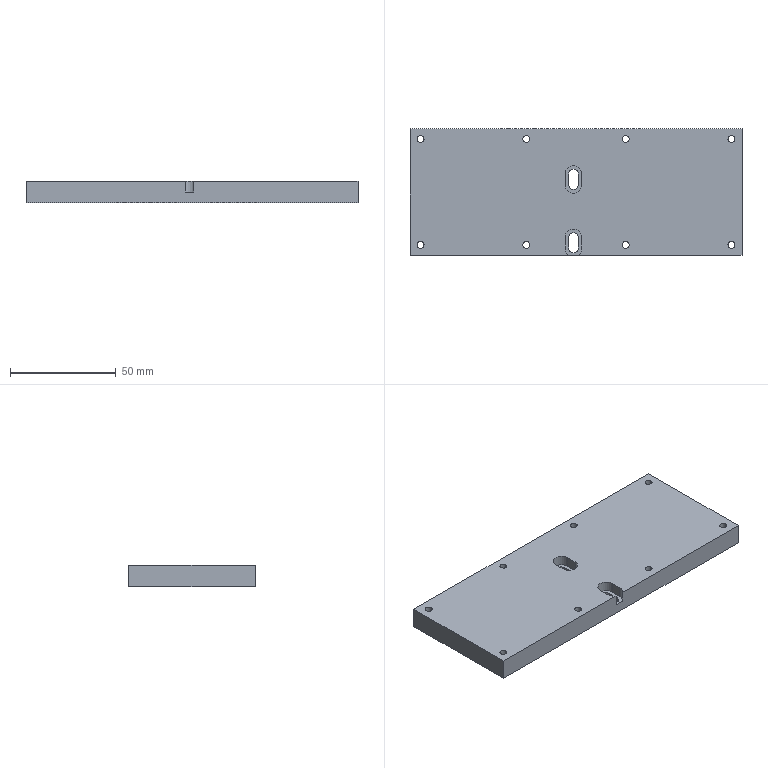Part | STEP file | 04-02-05 adjustment platform base plate | 1 solid | 41 faces | box 157 x 60 x 10 mm | volume 92232 mm3 | cylinder 25 | plane 16 | commonest cylinder face diameters 3.3 x16 8 x5 4.5 x4
STEP:
#1=CARTESIAN_POINT('',(71.85,25.,0.));
#2=VERTEX_POINT('',#1);
#3=CARTESIAN_POINT('',(75.15,25.,0.));
#4=VERTEX_POINT('',#3);
#5=CARTESIAN_POINT('',(73.5,25.,0.));
#6=DIRECTION('',(0.,0.,1.));
#7=DIRECTION('',(1.,0.,0.));
#8=AXIS2_PLACEMENT_3D('',#5,#6,#7);
#9=CIRCLE('',#8,1.65);
#10=EDGE_CURVE('',#2,#4,#9,.T.);
#11=ORIENTED_EDGE('',*,*,#10,.F.);
#12=CARTESIAN_POINT('',(71.85,25.,10.));
#13=VERTEX_POINT('',#12);
#14=CARTESIAN_POINT('',(71.85,25.,10.));
#15=DIRECTION('',(0.,0.,1.));
#16=VECTOR('',#15,1000.);
#17=LINE('',#14,#16);
#18=EDGE_CURVE('',#2,#13,#17,.T.);
#19=ORIENTED_EDGE('',*,*,#18,.T.);
#20=CARTESIAN_POINT('',(75.15,25.,10.));
#21=VERTEX_POINT('',#20);
#22=CARTESIAN_POINT('',(73.5,25.,10.));
#23=DIRECTION('',(0.,0.,1.));
#24=DIRECTION('',(1.,0.,0.));
#25=AXIS2_PLACEMENT_3D('',#22,#23,#24);
#26=CIRCLE('',#25,1.65);
#27=EDGE_CURVE('',#13,#21,#26,.T.);
#28=ORIENTED_EDGE('',*,*,#27,.T.);
#29=CARTESIAN_POINT('',(75.15,25.,10.));
#30=DIRECTION('',(0.,0.,1.));
#31=VECTOR('',#30,1000.);
#32=LINE('',#29,#31);
#33=EDGE_CURVE('',#4,#21,#32,.T.);
#34=ORIENTED_EDGE('',*,*,#33,.F.);
#35=EDGE_LOOP('',(#11,#19,#28,#34));
#36=FACE_OUTER_BOUND('',#35,.T.);
#37=CARTESIAN_POINT('',(73.5,25.,10.));
#38=DIRECTION('',(0.,0.,1.));
#39=DIRECTION('',(1.,0.,0.));
#40=AXIS2_PLACEMENT_3D('',#37,#38,#39);
#41=CYLINDRICAL_SURFACE('',#40,1.65);
#42=ADVANCED_FACE('',(#36),#41,.F.);
#43=CARTESIAN_POINT('',(21.85,-25.,0.));
#44=VERTEX_POINT('',#43);
#45=CARTESIAN_POINT('',(25.15,-25.,0.));
#46=VERTEX_POINT('',#45);
#47=CARTESIAN_POINT('',(23.5,-25.,0.));
#48=DIRECTION('',(0.,0.,1.));
#49=DIRECTION('',(1.,0.,0.));
#50=AXIS2_PLACEMENT_3D('',#47,#48,#49);
#51=CIRCLE('',#50,1.65);
#52=EDGE_CURVE('',#44,#46,#51,.T.);
#53=ORIENTED_EDGE('',*,*,#52,.F.);
#54=CARTESIAN_POINT('',(21.85,-25.,10.));
#55=VERTEX_POINT('',#54);
#56=CARTESIAN_POINT('',(21.85,-25.,10.));
#57=DIRECTION('',(0.,0.,1.));
#58=VECTOR('',#57,1000.);
#59=LINE('',#56,#58);
#60=EDGE_CURVE('',#44,#55,#59,.T.);
#61=ORIENTED_EDGE('',*,*,#60,.T.);
#62=CARTESIAN_POINT('',(25.15,-25.,10.));
#63=VERTEX_POINT('',#62);
#64=CARTESIAN_POINT('',(23.5,-25.,10.));
#65=DIRECTION('',(0.,0.,1.));
#66=DIRECTION('',(1.,0.,0.));
#67=AXIS2_PLACEMENT_3D('',#64,#65,#66);
#68=CIRCLE('',#67,1.65);
#69=EDGE_CURVE('',#55,#63,#68,.T.);
#70=ORIENTED_EDGE('',*,*,#69,.T.);
#71=CARTESIAN_POINT('',(25.15,-25.,10.));
#72=DIRECTION('',(0.,0.,1.));
#73=VECTOR('',#72,1000.);
#74=LINE('',#71,#73);
#75=EDGE_CURVE('',#46,#63,#74,.T.);
#76=ORIENTED_EDGE('',*,*,#75,.F.);
#77=EDGE_LOOP('',(#53,#61,#70,#76));
#78=FACE_OUTER_BOUND('',#77,.T.);
#79=CARTESIAN_POINT('',(23.5,-25.,10.));
#80=DIRECTION('',(0.,0.,1.));
#81=DIRECTION('',(1.,0.,0.));
#82=AXIS2_PLACEMENT_3D('',#79,#80,#81);
#83=CYLINDRICAL_SURFACE('',#82,1.65);
#84=ADVANCED_FACE('',(#78),#83,.F.);
#85=CARTESIAN_POINT('',(71.85,-25.,0.));
#86=VERTEX_POINT('',#85);
#87=CARTESIAN_POINT('',(75.15,-25.,0.));
#88=VERTEX_POINT('',#87);
#89=CARTESIAN_POINT('',(73.5,-25.,0.));
#90=DIRECTION('',(0.,0.,1.));
#91=DIRECTION('',(1.,0.,0.));
#92=AXIS2_PLACEMENT_3D('',#89,#90,#91);
#93=CIRCLE('',#92,1.65);
#94=EDGE_CURVE('',#86,#88,#93,.T.);
#95=ORIENTED_EDGE('',*,*,#94,.F.);
#96=CARTESIAN_POINT('',(71.85,-25.,10.));
#97=VERTEX_POINT('',#96);
#98=CARTESIAN_POINT('',(71.85,-25.,10.));
#99=DIRECTION('',(0.,0.,1.));
#100=VECTOR('',#99,1000.);
#101=LINE('',#98,#100);
#102=EDGE_CURVE('',#86,#97,#101,.T.);
#103=ORIENTED_EDGE('',*,*,#102,.T.);
#104=CARTESIAN_POINT('',(75.15,-25.,10.));
#105=VERTEX_POINT('',#104);
#106=CARTESIAN_POINT('',(73.5,-25.,10.));
#107=DIRECTION('',(0.,0.,1.));
#108=DIRECTION('',(1.,0.,0.));
#109=AXIS2_PLACEMENT_3D('',#106,#107,#108);
#110=CIRCLE('',#109,1.65);
#111=EDGE_CURVE('',#97,#105,#110,.T.);
#112=ORIENTED_EDGE('',*,*,#111,.T.);
#113=CARTESIAN_POINT('',(75.15,-25.,10.));
#114=DIRECTION('',(0.,0.,1.));
#115=VECTOR('',#114,1000.);
#116=LINE('',#113,#115);
#117=EDGE_CURVE('',#88,#105,#116,.T.);
#118=ORIENTED_EDGE('',*,*,#117,.F.);
#119=EDGE_LOOP('',(#95,#103,#112,#118));
#120=FACE_OUTER_BOUND('',#119,.T.);
#121=CARTESIAN_POINT('',(73.5,-25.,10.));
#122=DIRECTION('',(0.,0.,1.));
#123=DIRECTION('',(1.,0.,0.));
#124=AXIS2_PLACEMENT_3D('',#121,#122,#123);
#125=CYLINDRICAL_SURFACE('',#124,1.65);
#126=ADVANCED_FACE('',(#120),#125,.F.);
#127=CARTESIAN_POINT('',(21.85,25.,0.));
#128=VERTEX_POINT('',#127);
#129=CARTESIAN_POINT('',(25.15,25.,0.));
#130=VERTEX_POINT('',#129);
#131=CARTESIAN_POINT('',(23.5,25.,0.));
#132=DIRECTION('',(0.,0.,1.));
#133=DIRECTION('',(1.,0.,0.));
#134=AXIS2_PLACEMENT_3D('',#131,#132,#133);
#135=CIRCLE('',#134,1.65);
#136=EDGE_CURVE('',#128,#130,#135,.T.);
#137=ORIENTED_EDGE('',*,*,#136,.F.);
#138=CARTESIAN_POINT('',(21.85,25.,10.));
#139=VERTEX_POINT('',#138);
#140=CARTESIAN_POINT('',(21.85,25.,10.));
#141=DIRECTION('',(0.,0.,1.));
#142=VECTOR('',#141,1000.);
#143=LINE('',#140,#142);
#144=EDGE_CURVE('',#128,#139,#143,.T.);
#145=ORIENTED_EDGE('',*,*,#144,.T.);
#146=CARTESIAN_POINT('',(25.15,25.,10.));
#147=VERTEX_POINT('',#146);
#148=CARTESIAN_POINT('',(23.5,25.,10.));
#149=DIRECTION('',(0.,0.,1.));
#150=DIRECTION('',(1.,0.,0.));
#151=AXIS2_PLACEMENT_3D('',#148,#149,#150);
#152=CIRCLE('',#151,1.65);
#153=EDGE_CURVE('',#139,#147,#152,.T.);
#154=ORIENTED_EDGE('',*,*,#153,.T.);
#155=CARTESIAN_POINT('',(25.15,25.,10.));
#156=DIRECTION('',(0.,0.,1.));
#157=VECTOR('',#156,1000.);
#158=LINE('',#155,#157);
#159=EDGE_CURVE('',#130,#147,#158,.T.);
#160=ORIENTED_EDGE('',*,*,#159,.F.);
#161=EDGE_LOOP('',(#137,#145,#154,#160));
#162=FACE_OUTER_BOUND('',#161,.T.);
#163=CARTESIAN_POINT('',(23.5,25.,10.));
#164=DIRECTION('',(0.,0.,1.));
#165=DIRECTION('',(1.,0.,0.));
#166=AXIS2_PLACEMENT_3D('',#163,#164,#165);
#167=CYLINDRICAL_SURFACE('',#166,1.65);
#168=ADVANCED_FACE('',(#162),#167,.F.);
#169=CARTESIAN_POINT('',(-75.15,25.,0.));
#170=VERTEX_POINT('',#169);
#171=CARTESIAN_POINT('',(-71.85,25.,0.));
#172=VERTEX_POINT('',#171);
#173=CARTESIAN_POINT('',(-73.5,25.,0.));
#174=DIRECTION('',(0.,0.,1.));
#175=DIRECTION('',(1.,0.,0.));
#176=AXIS2_PLACEMENT_3D('',#173,#174,#175);
#177=CIRCLE('',#176,1.65);
#178=EDGE_CURVE('',#170,#172,#177,.T.);
#179=ORIENTED_EDGE('',*,*,#178,.F.);
#180=CARTESIAN_POINT('',(-75.15,25.,10.));
#181=VERTEX_POINT('',#180);
#182=CARTESIAN_POINT('',(-75.15,25.,10.));
#183=DIRECTION('',(0.,0.,1.));
#184=VECTOR('',#183,1000.);
#185=LINE('',#182,#184);
#186=EDGE_CURVE('',#170,#181,#185,.T.);
#187=ORIENTED_EDGE('',*,*,#186,.T.);
#188=CARTESIAN_POINT('',(-71.85,25.,10.));
#189=VERTEX_POINT('',#188);
#190=CARTESIAN_POINT('',(-73.5,25.,10.));
#191=DIRECTION('',(0.,0.,1.));
#192=DIRECTION('',(1.,0.,0.));
#193=AXIS2_PLACEMENT_3D('',#190,#191,#192);
#194=CIRCLE('',#193,1.65);
#195=EDGE_CURVE('',#181,#189,#194,.T.);
#196=ORIENTED_EDGE('',*,*,#195,.T.);
#197=CARTESIAN_POINT('',(-71.85,25.,10.));
#198=DIRECTION('',(0.,0.,1.));
#199=VECTOR('',#198,1000.);
#200=LINE('',#197,#199);
#201=EDGE_CURVE('',#172,#189,#200,.T.);
#202=ORIENTED_EDGE('',*,*,#201,.F.);
#203=EDGE_LOOP('',(#179,#187,#196,#202));
#204=FACE_OUTER_BOUND('',#203,.T.);
#205=CARTESIAN_POINT('',(-73.5,25.,10.));
#206=DIRECTION('',(0.,0.,1.));
#207=DIRECTION('',(1.,0.,0.));
#208=AXIS2_PLACEMENT_3D('',#205,#206,#207);
#209=CYLINDRICAL_SURFACE('',#208,1.65);
#210=ADVANCED_FACE('',(#204),#209,.F.);
#211=CARTESIAN_POINT('',(-25.15,25.,0.));
#212=VERTEX_POINT('',#211);
#213=CARTESIAN_POINT('',(-21.85,25.,0.));
#214=VERTEX_POINT('',#213);
#215=CARTESIAN_POINT('',(-23.5,25.,0.));
#216=DIRECTION('',(0.,0.,1.));
#217=DIRECTION('',(1.,0.,0.));
#218=AXIS2_PLACEMENT_3D('',#215,#216,#217);
#219=CIRCLE('',#218,1.65);
#220=EDGE_CURVE('',#212,#214,#219,.T.);
#221=ORIENTED_EDGE('',*,*,#220,.F.);
#222=CARTESIAN_POINT('',(-25.15,25.,10.));
#223=VERTEX_POINT('',#222);
#224=CARTESIAN_POINT('',(-25.15,25.,10.));
#225=DIRECTION('',(0.,0.,1.));
#226=VECTOR('',#225,1000.);
#227=LINE('',#224,#226);
#228=EDGE_CURVE('',#212,#223,#227,.T.);
#229=ORIENTED_EDGE('',*,*,#228,.T.);
#230=CARTESIAN_POINT('',(-21.85,25.,10.));
#231=VERTEX_POINT('',#230);
#232=CARTESIAN_POINT('',(-23.5,25.,10.));
#233=DIRECTION('',(0.,0.,1.));
#234=DIRECTION('',(1.,0.,0.));
#235=AXIS2_PLACEMENT_3D('',#232,#233,#234);
#236=CIRCLE('',#235,1.65);
#237=EDGE_CURVE('',#223,#231,#236,.T.);
#238=ORIENTED_EDGE('',*,*,#237,.T.);
#239=CARTESIAN_POINT('',(-21.85,25.,10.));
#240=DIRECTION('',(0.,0.,1.));
#241=VECTOR('',#240,1000.);
#242=LINE('',#239,#241);
#243=EDGE_CURVE('',#214,#231,#242,.T.);
#244=ORIENTED_EDGE('',*,*,#243,.F.);
#245=EDGE_LOOP('',(#221,#229,#238,#244));
#246=FACE_OUTER_BOUND('',#245,.T.);
#247=CARTESIAN_POINT('',(-23.5,25.,10.));
#248=DIRECTION('',(0.,0.,1.));
#249=DIRECTION('',(1.,0.,0.));
#250=AXIS2_PLACEMENT_3D('',#247,#248,#249);
#251=CYLINDRICAL_SURFACE('',#250,1.65);
#252=ADVANCED_FACE('',(#246),#251,.F.);
#253=CARTESIAN_POINT('',(-75.15,-25.,0.));
#254=VERTEX_POINT('',#253);
#255=CARTESIAN_POINT('',(-71.85,-25.,0.));
#256=VERTEX_POINT('',#255);
#257=CARTESIAN_POINT('',(-73.5,-25.,0.));
#258=DIRECTION('',(0.,0.,1.));
#259=DIRECTION('',(1.,0.,0.));
#260=AXIS2_PLACEMENT_3D('',#257,#258,#259);
#261=CIRCLE('',#260,1.65);
#262=EDGE_CURVE('',#254,#256,#261,.T.);
#263=ORIENTED_EDGE('',*,*,#262,.F.);
#264=CARTESIAN_POINT('',(-75.15,-25.,10.));
#265=VERTEX_POINT('',#264);
#266=CARTESIAN_POINT('',(-75.15,-25.,10.));
#267=DIRECTION('',(0.,0.,1.));
#268=VECTOR('',#267,1000.);
#269=LINE('',#266,#268);
#270=EDGE_CURVE('',#254,#265,#269,.T.);
#271=ORIENTED_EDGE('',*,*,#270,.T.);
#272=CARTESIAN_POINT('',(-71.85,-25.,10.));
#273=VERTEX_POINT('',#272);
#274=CARTESIAN_POINT('',(-73.5,-25.,10.));
#275=DIRECTION('',(0.,0.,1.));
#276=DIRECTION('',(1.,0.,0.));
#277=AXIS2_PLACEMENT_3D('',#274,#275,#276);
#278=CIRCLE('',#277,1.65);
#279=EDGE_CURVE('',#265,#273,#278,.T.);
#280=ORIENTED_EDGE('',*,*,#279,.T.);
#281=CARTESIAN_POINT('',(-71.85,-25.,10.));
#282=DIRECTION('',(0.,0.,1.));
#283=VECTOR('',#282,1000.);
#284=LINE('',#281,#283);
#285=EDGE_CURVE('',#256,#273,#284,.T.);
#286=ORIENTED_EDGE('',*,*,#285,.F.);
#287=EDGE_LOOP('',(#263,#271,#280,#286));
#288=FACE_OUTER_BOUND('',#287,.T.);
#289=CARTESIAN_POINT('',(-73.5,-25.,10.));
#290=DIRECTION('',(0.,0.,1.));
#291=DIRECTION('',(1.,0.,0.));
#292=AXIS2_PLACEMENT_3D('',#289,#290,#291);
#293=CYLINDRICAL_SURFACE('',#292,1.65);
#294=ADVANCED_FACE('',(#288),#293,.F.);
#295=CARTESIAN_POINT('',(-25.15,-25.,0.));
#296=VERTEX_POINT('',#295);
#297=CARTESIAN_POINT('',(-21.85,-25.,0.));
#298=VERTEX_POINT('',#297);
#299=CARTESIAN_POINT('',(-23.5,-25.,0.));
#300=DIRECTION('',(0.,0.,1.));
#301=DIRECTION('',(1.,0.,0.));
#302=AXIS2_PLACEMENT_3D('',#299,#300,#301);
#303=CIRCLE('',#302,1.65);
#304=EDGE_CURVE('',#296,#298,#303,.T.);
#305=ORIENTED_EDGE('',*,*,#304,.F.);
#306=CARTESIAN_POINT('',(-25.15,-25.,10.));
#307=VERTEX_POINT('',#306);
#308=CARTESIAN_POINT('',(-25.15,-25.,10.));
#309=DIRECTION('',(0.,0.,1.));
#310=VECTOR('',#309,1000.);
#311=LINE('',#308,#310);
#312=EDGE_CURVE('',#296,#307,#311,.T.);
#313=ORIENTED_EDGE('',*,*,#312,.T.);
#314=CARTESIAN_POINT('',(-21.85,-25.,10.));
#315=VERTEX_POINT('',#314);
#316=CARTESIAN_POINT('',(-23.5,-25.,10.));
#317=DIRECTION('',(0.,0.,1.));
#318=DIRECTION('',(1.,0.,0.));
#319=AXIS2_PLACEMENT_3D('',#316,#317,#318);
#320=CIRCLE('',#319,1.65);
#321=EDGE_CURVE('',#307,#315,#320,.T.);
#322=ORIENTED_EDGE('',*,*,#321,.T.);
#323=CARTESIAN_POINT('',(-21.85,-25.,10.));
#324=DIRECTION('',(0.,0.,1.));
#325=VECTOR('',#324,1000.);
#326=LINE('',#323,#325);
#327=EDGE_CURVE('',#298,#315,#326,.T.);
#328=ORIENTED_EDGE('',*,*,#327,.F.);
#329=EDGE_LOOP('',(#305,#313,#322,#328));
#330=FACE_OUTER_BOUND('',#329,.T.);
#331=CARTESIAN_POINT('',(-23.5,-25.,10.));
#332=DIRECTION('',(0.,0.,1.));
#333=DIRECTION('',(1.,0.,0.));
#334=AXIS2_PLACEMENT_3D('',#331,#332,#333);
#335=CYLINDRICAL_SURFACE('',#334,1.65);
#336=ADVANCED_FACE('',(#330),#335,.F.);
#337=CARTESIAN_POINT('',(-3.45,-21.5,5.));
#338=VERTEX_POINT('',#337);
#339=CARTESIAN_POINT('',(1.05,-21.5,5.));
#340=VERTEX_POINT('',#339);
#341=CARTESIAN_POINT('',(-1.2,-21.5,5.));
#342=DIRECTION('',(0.,0.,-1.));
#343=DIRECTION('',(1.,0.,0.));
#344=AXIS2_PLACEMENT_3D('',#341,#342,#343);
#345=CIRCLE('',#344,2.25);
#346=EDGE_CURVE('',#338,#340,#345,.T.);
#347=ORIENTED_EDGE('',*,*,#346,.F.);
#348=CARTESIAN_POINT('',(-3.45,-21.5,0.));
#349=VERTEX_POINT('',#348);
#350=CARTESIAN_POINT('',(-3.45,-21.5,0.));
#351=DIRECTION('',(0.,0.,1.));
#352=VECTOR('',#351,1000.);
#353=LINE('',#350,#352);
#354=EDGE_CURVE('',#349,#338,#353,.T.);
#355=ORIENTED_EDGE('',*,*,#354,.F.);
#356=CARTESIAN_POINT('',(1.05,-21.5,0.));
#357=VERTEX_POINT('',#356);
#358=CARTESIAN_POINT('',(-1.2,-21.5,0.));
#359=DIRECTION('',(0.,0.,1.));
#360=DIRECTION('',(1.,0.,0.));
#361=AXIS2_PLACEMENT_3D('',#358,#359,#360);
#362=CIRCLE('',#361,2.25);
#363=EDGE_CURVE('',#357,#349,#362,.T.);
#364=ORIENTED_EDGE('',*,*,#363,.F.);
#365=CARTESIAN_POINT('',(1.05,-21.5,0.));
#366=DIRECTION('',(0.,0.,1.));
#367=VECTOR('',#366,1000.);
#368=LINE('',#365,#367);
#369=EDGE_CURVE('',#357,#340,#368,.T.);
#370=ORIENTED_EDGE('',*,*,#369,.T.);
#371=EDGE_LOOP('',(#347,#355,#364,#370));
#372=FACE_OUTER_BOUND('',#371,.T.);
#373=CARTESIAN_POINT('',(-1.2,-21.5,0.));
#374=DIRECTION('',(0.,0.,1.));
#375=DIRECTION('',(1.,0.,0.));
#376=AXIS2_PLACEMENT_3D('',#373,#374,#375);
#377=CYLINDRICAL_SURFACE('',#376,2.25);
#378=ADVANCED_FACE('',(#372),#377,.F.);
#379=CARTESIAN_POINT('',(1.05,-26.5,5.));
#380=VERTEX_POINT('',#379);
#381=CARTESIAN_POINT('',(1.05,-21.5,5.));
#382=DIRECTION('',(0.,-1.,0.));
#383=VECTOR('',#382,1000.);
#384=LINE('',#381,#383);
#385=EDGE_CURVE('',#340,#380,#384,.T.);
#386=ORIENTED_EDGE('',*,*,#385,.F.);
#387=ORIENTED_EDGE('',*,*,#369,.F.);
#388=CARTESIAN_POINT('',(1.05,-26.5,0.));
#389=VERTEX_POINT('',#388);
#390=CARTESIAN_POINT('',(1.05,-21.5,0.));
#391=DIRECTION('',(0.,1.,0.));
#392=VECTOR('',#391,1000.);
#393=LINE('',#390,#392);
#394=EDGE_CURVE('',#389,#357,#393,.T.);
#395=ORIENTED_EDGE('',*,*,#394,.F.);
#396=CARTESIAN_POINT('',(1.05,-26.5,0.));
#397=DIRECTION('',(0.,0.,1.));
#398=VECTOR('',#397,1000.);
#399=LINE('',#396,#398);
#400=EDGE_CURVE('',#389,#380,#399,.T.);
#401=ORIENTED_EDGE('',*,*,#400,.T.);
#402=EDGE_LOOP('',(#386,#387,#395,#401));
#403=FACE_OUTER_BOUND('',#402,.T.);
#404=CARTESIAN_POINT('',(1.05,-21.5,0.));
#405=DIRECTION('',(1.,0.,0.));
#406=DIRECTION('',(0.,1.,0.));
#407=AXIS2_PLACEMENT_3D('',#404,#405,#406);
#408=PLANE('',#407);
#409=ADVANCED_FACE('',(#403),#408,.F.);
#410=CARTESIAN_POINT('',(-3.45,-26.5,5.));
#411=VERTEX_POINT('',#410);
#412=CARTESIAN_POINT('',(-1.2,-26.5,5.));
#413=DIRECTION('',(0.,0.,-1.));
#414=DIRECTION('',(1.,0.,0.));
#415=AXIS2_PLACEMENT_3D('',#412,#413,#414);
#416=CIRCLE('',#415,2.25);
#417=EDGE_CURVE('',#380,#411,#416,.T.);
#418=ORIENTED_EDGE('',*,*,#417,.F.);
#419=ORIENTED_EDGE('',*,*,#400,.F.);
#420=CARTESIAN_POINT('',(-3.45,-26.5,0.));
#421=VERTEX_POINT('',#420);
#422=CARTESIAN_POINT('',(-1.2,-26.5,0.));
#423=DIRECTION('',(0.,0.,1.));
#424=DIRECTION('',(1.,0.,0.));
#425=AXIS2_PLACEMENT_3D('',#422,#423,#424);
#426=CIRCLE('',#425,2.25);
#427=EDGE_CURVE('',#421,#389,#426,.T.);
#428=ORIENTED_EDGE('',*,*,#427,.F.);
#429=CARTESIAN_POINT('',(-3.45,-26.5,0.));
#430=DIRECTION('',(0.,0.,1.));
#431=VECTOR('',#430,1000.);
#432=LINE('',#429,#431);
#433=EDGE_CURVE('',#421,#411,#432,.T.);
#434=ORIENTED_EDGE('',*,*,#433,.T.);
#435=EDGE_LOOP('',(#418,#419,#428,#434));
#436=FACE_OUTER_BOUND('',#435,.T.);
#437=CARTESIAN_POINT('',(-1.2,-26.5,0.));
#438=DIRECTION('',(0.,0.,1.));
#439=DIRECTION('',(1.,0.,0.));
#440=AXIS2_PLACEMENT_3D('',#437,#438,#439);
#441=CYLINDRICAL_SURFACE('',#440,2.25);
#442=ADVANCED_FACE('',(#436),#441,.F.);
#443=CARTESIAN_POINT('',(-3.45,-21.5,5.));
#444=DIRECTION('',(0.,1.,0.));
#445=VECTOR('',#444,1000.);
#446=LINE('',#443,#445);
#447=EDGE_CURVE('',#411,#338,#446,.T.);
#448=ORIENTED_EDGE('',*,*,#447,.F.);
#449=ORIENTED_EDGE('',*,*,#433,.F.);
#450=CARTESIAN_POINT('',(-3.45,-21.5,0.));
#451=DIRECTION('',(0.,-1.,0.));
#452=VECTOR('',#451,1000.);
#453=LINE('',#450,#452);
#454=EDGE_CURVE('',#349,#421,#453,.T.);
#455=ORIENTED_EDGE('',*,*,#454,.F.);
#456=ORIENTED_EDGE('',*,*,#354,.T.);
#457=EDGE_LOOP('',(#448,#449,#455,#456));
#458=FACE_OUTER_BOUND('',#457,.T.);
#459=CARTESIAN_POINT('',(-3.45,-21.5,0.));
#460=DIRECTION('',(-1.,0.,0.));
#461=DIRECTION('',(0.,-1.,0.));
#462=AXIS2_PLACEMENT_3D('',#459,#460,#461);
#463=PLANE('',#462);
#464=ADVANCED_FACE('',(#458),#463,.F.);
#465=CARTESIAN_POINT('',(-3.45,8.5,5.));
#466=VERTEX_POINT('',#465);
#467=CARTESIAN_POINT('',(1.05,8.5,5.));
#468=VERTEX_POINT('',#467);
#469=CARTESIAN_POINT('',(-1.2,8.5,5.));
#470=DIRECTION('',(0.,0.,-1.));
#471=DIRECTION('',(1.,0.,0.));
#472=AXIS2_PLACEMENT_3D('',#469,#470,#471);
#473=CIRCLE('',#472,2.25);
#474=EDGE_CURVE('',#466,#468,#473,.T.);
#475=ORIENTED_EDGE('',*,*,#474,.F.);
#476=CARTESIAN_POINT('',(-3.45,8.5,0.));
#477=VERTEX_POINT('',#476);
#478=CARTESIAN_POINT('',(-3.45,8.5,0.));
#479=DIRECTION('',(0.,0.,1.));
#480=VECTOR('',#479,1000.);
#481=LINE('',#478,#480);
#482=EDGE_CURVE('',#477,#466,#481,.T.);
#483=ORIENTED_EDGE('',*,*,#482,.F.);
#484=CARTESIAN_POINT('',(1.05,8.5,0.));
#485=VERTEX_POINT('',#484);
#486=CARTESIAN_POINT('',(-1.2,8.5,0.));
#487=DIRECTION('',(0.,0.,1.));
#488=DIRECTION('',(1.,0.,0.));
#489=AXIS2_PLACEMENT_3D('',#486,#487,#488);
#490=CIRCLE('',#489,2.25);
#491=EDGE_CURVE('',#485,#477,#490,.T.);
#492=ORIENTED_EDGE('',*,*,#491,.F.);
#493=CARTESIAN_POINT('',(1.05,8.5,0.));
#494=DIRECTION('',(0.,0.,1.));
#495=VECTOR('',#494,1000.);
#496=LINE('',#493,#495);
#497=EDGE_CURVE('',#485,#468,#496,.T.);
#498=ORIENTED_EDGE('',*,*,#497,.T.);
#499=EDGE_LOOP('',(#475,#483,#492,#498));
#500=FACE_OUTER_BOUND('',#499,.T.);
#501=CARTESIAN_POINT('',(-1.2,8.5,0.));
#502=DIRECTION('',(0.,0.,1.));
#503=DIRECTION('',(1.,0.,0.));
#504=AXIS2_PLACEMENT_3D('',#501,#502,#503);
#505=CYLINDRICAL_SURFACE('',#504,2.25);
#506=ADVANCED_FACE('',(#500),#505,.F.);
#507=CARTESIAN_POINT('',(1.05,3.5,5.));
#508=VERTEX_POINT('',#507);
#509=CARTESIAN_POINT('',(1.05,8.5,5.));
#510=DIRECTION('',(0.,-1.,0.));
#511=VECTOR('',#510,1000.);
#512=LINE('',#509,#511);
#513=EDGE_CURVE('',#468,#508,#512,.T.);
#514=ORIENTED_EDGE('',*,*,#513,.F.);
#515=ORIENTED_EDGE('',*,*,#497,.F.);
#516=CARTESIAN_POINT('',(1.05,3.5,0.));
#517=VERTEX_POINT('',#516);
#518=CARTESIAN_POINT('',(1.05,8.5,0.));
#519=DIRECTION('',(0.,1.,0.));
#520=VECTOR('',#519,1000.);
#521=LINE('',#518,#520);
#522=EDGE_CURVE('',#517,#485,#521,.T.);
#523=ORIENTED_EDGE('',*,*,#522,.F.);
#524=CARTESIAN_POINT('',(1.05,3.5,0.));
#525=DIRECTION('',(0.,0.,1.));
#526=VECTOR('',#525,1000.);
#527=LINE('',#524,#526);
#528=EDGE_CURVE('',#517,#508,#527,.T.);
#529=ORIENTED_EDGE('',*,*,#528,.T.);
#530=EDGE_LOOP('',(#514,#515,#523,#529));
#531=FACE_OUTER_BOUND('',#530,.T.);
#532=CARTESIAN_POINT('',(1.05,8.5,0.));
#533=DIRECTION('',(1.,0.,0.));
#534=DIRECTION('',(0.,1.,0.));
#535=AXIS2_PLACEMENT_3D('',#532,#533,#534);
#536=PLANE('',#535);
#537=ADVANCED_FACE('',(#531),#536,.F.);
#538=CARTESIAN_POINT('',(-3.45,3.5,5.));
#539=VERTEX_POINT('',#538);
#540=CARTESIAN_POINT('',(-1.2,3.5,5.));
#541=DIRECTION('',(0.,0.,-1.));
#542=DIRECTION('',(1.,0.,0.));
#543=AXIS2_PLACEMENT_3D('',#540,#541,#542);
#544=CIRCLE('',#543,2.25);
#545=EDGE_CURVE('',#508,#539,#544,.T.);
#546=ORIENTED_EDGE('',*,*,#545,.F.);
#547=ORIENTED_EDGE('',*,*,#528,.F.);
#548=CARTESIAN_POINT('',(-3.45,3.5,0.));
#549=VERTEX_POINT('',#548);
#550=CARTESIAN_POINT('',(-1.2,3.5,0.));
#551=DIRECTION('',(0.,0.,1.));
#552=DIRECTION('',(1.,0.,0.));
#553=AXIS2_PLACEMENT_3D('',#550,#551,#552);
#554=CIRCLE('',#553,2.25);
#555=EDGE_CURVE('',#549,#517,#554,.T.);
#556=ORIENTED_EDGE('',*,*,#555,.F.);
#557=CARTESIAN_POINT('',(-3.45,3.5,0.));
#558=DIRECTION('',(0.,0.,1.));
#559=VECTOR('',#558,1000.);
#560=LINE('',#557,#559);
#561=EDGE_CURVE('',#549,#539,#560,.T.);
#562=ORIENTED_EDGE('',*,*,#561,.T.);
#563=EDGE_LOOP('',(#546,#547,#556,#562));
#564=FACE_OUTER_BOUND('',#563,.T.);
#565=CARTESIAN_POINT('',(-1.2,3.5,0.));
#566=DIRECTION('',(0.,0.,1.));
#567=DIRECTION('',(1.,0.,0.));
#568=AXIS2_PLACEMENT_3D('',#565,#566,#567);
#569=CYLINDRICAL_SURFACE('',#568,2.25);
#570=ADVANCED_FACE('',(#564),#569,.F.);
#571=CARTESIAN_POINT('',(-3.45,8.5,5.));
#572=DIRECTION('',(0.,1.,0.));
#573=VECTOR('',#572,1000.);
#574=LINE('',#571,#573);
#575=EDGE_CURVE('',#539,#466,#574,.T.);
#576=ORIENTED_EDGE('',*,*,#575,.F.);
#577=ORIENTED_EDGE('',*,*,#561,.F.);
#578=CARTESIAN_POINT('',(-3.45,8.5,0.));
#579=DIRECTION('',(0.,-1.,0.));
#580=VECTOR('',#579,1000.);
#581=LINE('',#578,#580);
#582=EDGE_CURVE('',#477,#549,#581,.T.);
#583=ORIENTED_EDGE('',*,*,#582,.F.);
#584=ORIENTED_EDGE('',*,*,#482,.T.);
#585=EDGE_LOOP('',(#576,#577,#583,#584));
#586=FACE_OUTER_BOUND('',#585,.T.);
#587=CARTESIAN_POINT('',(-3.45,8.5,0.));
#588=DIRECTION('',(-1.,0.,0.));
#589=DIRECTION('',(0.,-1.,0.));
#590=AXIS2_PLACEMENT_3D('',#587,#588,#589);
#591=PLANE('',#590);
#592=ADVANCED_FACE('',(#586),#591,.F.);
#593=CARTESIAN_POINT('',(78.5,-30.,0.));
#594=VERTEX_POINT('',#593);
#595=CARTESIAN_POINT('',(78.5,30.,0.));
#596=VERTEX_POINT('',#595);
#597=CARTESIAN_POINT('',(78.5,30.,0.));
#598=DIRECTION('',(0.,1.,0.));
#599=VECTOR('',#598,1000.);
#600=LINE('',#597,#599);
#601=EDGE_CURVE('',#594,#596,#600,.T.);
#602=ORIENTED_EDGE('',*,*,#601,.T.);
#603=CARTESIAN_POINT('',(78.5,30.,10.));
#604=VERTEX_POINT('',#603);
#605=CARTESIAN_POINT('',(78.5,30.,10.));
#606=DIRECTION('',(0.,0.,-1.));
#607=VECTOR('',#606,1000.);
#608=LINE('',#605,#607);
#609=EDGE_CURVE('',#604,#596,#608,.T.);
#610=ORIENTED_EDGE('',*,*,#609,.F.);
#611=CARTESIAN_POINT('',(78.5,-30.,10.));
#612=VERTEX_POINT('',#611);
#613=CARTESIAN_POINT('',(78.5,30.,10.));
#614=DIRECTION('',(0.,1.,0.));
#615=VECTOR('',#614,1000.);
#616=LINE('',#613,#615);
#617=EDGE_CURVE('',#612,#604,#616,.T.);
#618=ORIENTED_EDGE('',*,*,#617,.F.);
#619=CARTESIAN_POINT('',(78.5,-30.,10.));
#620=DIRECTION('',(0.,0.,-1.));
#621=VECTOR('',#620,1000.);
#622=LINE('',#619,#621);
#623=EDGE_CURVE('',#612,#594,#622,.T.);
#624=ORIENTED_EDGE('',*,*,#623,.T.);
#625=EDGE_LOOP('',(#602,#610,#618,#624));
#626=FACE_OUTER_BOUND('',#625,.T.);
#627=CARTESIAN_POINT('',(78.5,30.,10.));
#628=DIRECTION('',(-1.,0.,0.));
#629=DIRECTION('',(0.,-1.,0.));
#630=AXIS2_PLACEMENT_3D('',#627,#628,#629);
#631=PLANE('',#630);
#632=ADVANCED_FACE('',(#626),#631,.F.);
#633=CARTESIAN_POINT('',(-78.5,30.,0.));
#634=VERTEX_POINT('',#633);
#635=CARTESIAN_POINT('',(-78.5,30.,0.));
#636=DIRECTION('',(-1.,0.,0.));
#637=VECTOR('',#636,1000.);
#638=LINE('',#635,#637);
#639=EDGE_CURVE('',#596,#634,#638,.T.);
#640=ORIENTED_EDGE('',*,*,#639,.T.);
#641=CARTESIAN_POINT('',(-78.5,30.,10.));
#642=VERTEX_POINT('',#641);
#643=CARTESIAN_POINT('',(-78.5,30.,10.));
#644=DIRECTION('',(0.,0.,-1.));
#645=VECTOR('',#644,1000.);
#646=LINE('',#643,#645);
#647=EDGE_CURVE('',#642,#634,#646,.T.);
#648=ORIENTED_EDGE('',*,*,#647,.F.);
#649=CARTESIAN_POINT('',(-78.5,30.,10.));
#650=DIRECTION('',(-1.,0.,0.));
#651=VECTOR('',#650,1000.);
#652=LINE('',#649,#651);
#653=EDGE_CURVE('',#604,#642,#652,.T.);
#654=ORIENTED_EDGE('',*,*,#653,.F.);
#655=ORIENTED_EDGE('',*,*,#609,.T.);
#656=EDGE_LOOP('',(#640,#648,#654,#655));
#657=FACE_OUTER_BOUND('',#656,.T.);
#658=CARTESIAN_POINT('',(-78.5,30.,10.));
#659=DIRECTION('',(0.,-1.,0.));
#660=DIRECTION('',(0.,0.,-1.));
#661=AXIS2_PLACEMENT_3D('',#658,#659,#660);
#662=PLANE('',#661);
#663=ADVANCED_FACE('',(#657),#662,.F.);
#664=CARTESIAN_POINT('',(-78.5,-30.,0.));
#665=VERTEX_POINT('',#664);
#666=CARTESIAN_POINT('',(-78.5,30.,0.));
#667=DIRECTION('',(0.,-1.,0.));
#668=VECTOR('',#667,1000.);
#669=LINE('',#666,#668);
#670=EDGE_CURVE('',#634,#665,#669,.T.);
#671=ORIENTED_EDGE('',*,*,#670,.T.);
#672=CARTESIAN_POINT('',(-78.5,-30.,10.));
#673=VERTEX_POINT('',#672);
#674=CARTESIAN_POINT('',(-78.5,-30.,10.));
#675=DIRECTION('',(0.,0.,-1.));
#676=VECTOR('',#675,1000.);
#677=LINE('',#674,#676);
#678=EDGE_CURVE('',#673,#665,#677,.T.);
#679=ORIENTED_EDGE('',*,*,#678,.F.);
#680=CARTESIAN_POINT('',(-78.5,30.,10.));
#681=DIRECTION('',(0.,-1.,0.));
#682=VECTOR('',#681,1000.);
#683=LINE('',#680,#682);
#684=EDGE_CURVE('',#642,#673,#683,.T.);
#685=ORIENTED_EDGE('',*,*,#684,.F.);
#686=ORIENTED_EDGE('',*,*,#647,.T.);
#687=EDGE_LOOP('',(#671,#679,#685,#686));
#688=FACE_OUTER_BOUND('',#687,.T.);
#689=CARTESIAN_POINT('',(-78.5,30.,10.));
#690=DIRECTION('',(1.,0.,0.));
#691=DIRECTION('',(0.,1.,0.));
#692=AXIS2_PLACEMENT_3D('',#689,#690,#691);
#693=PLANE('',#692);
#694=ADVANCED_FACE('',(#688),#693,.F.);
#695=CARTESIAN_POINT('',(-3.247,-30.,5.));
#696=VERTEX_POINT('',#695);
#697=CARTESIAN_POINT('',(0.8468,-30.,5.));
#698=VERTEX_POINT('',#697);
#699=CARTESIAN_POINT('',(-78.5,-30.,5.));
#700=DIRECTION('',(1.,0.,0.));
#701=VECTOR('',#700,1000.);
#702=LINE('',#699,#701);
#703=EDGE_CURVE('',#696,#698,#702,.T.);
#704=ORIENTED_EDGE('',*,*,#703,.F.);
#705=CARTESIAN_POINT('',(-3.247,-30.,10.));
#706=VERTEX_POINT('',#705);
#707=CARTESIAN_POINT('',(-3.247,-30.,5.));
#708=DIRECTION('',(0.,0.,1.));
#709=VECTOR('',#708,1000.);
#710=LINE('',#707,#709);
#711=EDGE_CURVE('',#696,#706,#710,.T.);
#712=ORIENTED_EDGE('',*,*,#711,.T.);
#713=CARTESIAN_POINT('',(-78.5,-30.,10.));
#714=DIRECTION('',(1.,0.,0.));
#715=VECTOR('',#714,1000.);
#716=LINE('',#713,#715);
#717=EDGE_CURVE('',#673,#706,#716,.T.);
#718=ORIENTED_EDGE('',*,*,#717,.F.);
#719=ORIENTED_EDGE('',*,*,#678,.T.);
#720=CARTESIAN_POINT('',(-78.5,-30.,0.));
#721=DIRECTION('',(1.,0.,0.));
#722=VECTOR('',#721,1000.);
#723=LINE('',#720,#722);
#724=EDGE_CURVE('',#665,#594,#723,.T.);
#725=ORIENTED_EDGE('',*,*,#724,.T.);
#726=ORIENTED_EDGE('',*,*,#623,.F.);
#727=CARTESIAN_POINT('',(0.8468,-30.,10.));
#728=VERTEX_POINT('',#727);
#729=CARTESIAN_POINT('',(-78.5,-30.,10.));
#730=DIRECTION('',(1.,0.,0.));
#731=VECTOR('',#730,1000.);
#732=LINE('',#729,#731);
#733=EDGE_CURVE('',#728,#612,#732,.T.);
#734=ORIENTED_EDGE('',*,*,#733,.F.);
#735=CARTESIAN_POINT('',(0.8468,-30.,5.));
#736=DIRECTION('',(0.,0.,-1.));
#737=VECTOR('',#736,1000.);
#738=LINE('',#735,#737);
#739=EDGE_CURVE('',#728,#698,#738,.T.);
#740=ORIENTED_EDGE('',*,*,#739,.T.);
#741=EDGE_LOOP('',(#704,#712,#718,#719,#725,#726,#734,#740));
#742=FACE_OUTER_BOUND('',#741,.T.);
#743=CARTESIAN_POINT('',(-78.5,-30.,10.));
#744=DIRECTION('',(0.,1.,0.));
#745=DIRECTION('',(0.,0.,1.));
#746=AXIS2_PLACEMENT_3D('',#743,#744,#745);
#747=PLANE('',#746);
#748=ADVANCED_FACE('',(#742),#747,.F.);
#749=CARTESIAN_POINT('',(2.8,-26.563,10.));
#750=VERTEX_POINT('',#749);
#751=CARTESIAN_POINT('',(-1.2,-26.563,10.));
#752=DIRECTION('',(0.,0.,1.));
#753=DIRECTION('',(1.,0.,0.));
#754=AXIS2_PLACEMENT_3D('',#751,#752,#753);
#755=CIRCLE('',#754,4.);
#756=EDGE_CURVE('',#728,#750,#755,.T.);
#757=ORIENTED_EDGE('',*,*,#756,.F.);
#758=ORIENTED_EDGE('',*,*,#733,.T.);
#759=ORIENTED_EDGE('',*,*,#617,.T.);
#760=ORIENTED_EDGE('',*,*,#653,.T.);
#761=ORIENTED_EDGE('',*,*,#684,.T.);
#762=ORIENTED_EDGE('',*,*,#717,.T.);
#763=CARTESIAN_POINT('',(-5.2,-26.563,10.));
#764=VERTEX_POINT('',#763);
#765=CARTESIAN_POINT('',(-1.2,-26.563,10.));
#766=DIRECTION('',(0.,0.,1.));
#767=DIRECTION('',(1.,0.,0.));
#768=AXIS2_PLACEMENT_3D('',#765,#766,#767);
#769=CIRCLE('',#768,4.);
#770=EDGE_CURVE('',#764,#706,#769,.T.);
#771=ORIENTED_EDGE('',*,*,#770,.F.);
#772=CARTESIAN_POINT('',(-5.2,-21.5,10.));
#773=VERTEX_POINT('',#772);
#774=CARTESIAN_POINT('',(-5.2,-21.5,10.));
#775=DIRECTION('',(0.,-1.,0.));
#776=VECTOR('',#775,1000.);
#777=LINE('',#774,#776);
#778=EDGE_CURVE('',#773,#764,#777,.T.);
#779=ORIENTED_EDGE('',*,*,#778,.F.);
#780=CARTESIAN_POINT('',(2.8,-21.5,10.));
#781=VERTEX_POINT('',#780);
#782=CARTESIAN_POINT('',(-1.2,-21.5,10.));
#783=DIRECTION('',(0.,0.,1.));
#784=DIRECTION('',(1.,0.,0.));
#785=AXIS2_PLACEMENT_3D('',#782,#783,#784);
#786=CIRCLE('',#785,4.);
#787=EDGE_CURVE('',#781,#773,#786,.T.);
#788=ORIENTED_EDGE('',*,*,#787,.F.);
#789=CARTESIAN_POINT('',(2.8,-21.5,10.));
#790=DIRECTION('',(0.,1.,0.));
#791=VECTOR('',#790,1000.);
#792=LINE('',#789,#791);
#793=EDGE_CURVE('',#750,#781,#792,.T.);
#794=ORIENTED_EDGE('',*,*,#793,.F.);
#795=EDGE_LOOP('',(#757,#758,#759,#760,#761,#762,#771,#779,#788,#794));
#796=FACE_OUTER_BOUND('',#795,.T.);
#797=CARTESIAN_POINT('',(2.8,8.5,10.));
#798=VERTEX_POINT('',#797);
#799=CARTESIAN_POINT('',(-5.2,8.5,10.));
#800=VERTEX_POINT('',#799);
#801=CARTESIAN_POINT('',(-1.2,8.5,10.));
#802=DIRECTION('',(0.,0.,1.));
#803=DIRECTION('',(1.,0.,0.));
#804=AXIS2_PLACEMENT_3D('',#801,#802,#803);
#805=CIRCLE('',#804,4.);
#806=EDGE_CURVE('',#798,#800,#805,.T.);
#807=ORIENTED_EDGE('',*,*,#806,.F.);
#808=CARTESIAN_POINT('',(2.8,3.437,10.));
#809=VERTEX_POINT('',#808);
#810=CARTESIAN_POINT('',(2.8,8.5,10.));
#811=DIRECTION('',(0.,1.,0.));
#812=VECTOR('',#811,1000.);
#813=LINE('',#810,#812);
#814=EDGE_CURVE('',#809,#798,#813,.T.);
#815=ORIENTED_EDGE('',*,*,#814,.F.);
#816=CARTESIAN_POINT('',(-5.2,3.437,10.));
#817=VERTEX_POINT('',#816);
#818=CARTESIAN_POINT('',(-1.2,3.437,10.));
#819=DIRECTION('',(0.,0.,1.));
#820=DIRECTION('',(1.,0.,0.));
#821=AXIS2_PLACEMENT_3D('',#818,#819,#820);
#822=CIRCLE('',#821,4.);
#823=EDGE_CURVE('',#817,#809,#822,.T.);
#824=ORIENTED_EDGE('',*,*,#823,.F.);
#825=CARTESIAN_POINT('',(-5.2,8.5,10.));
#826=DIRECTION('',(0.,-1.,0.));
#827=VECTOR('',#826,1000.);
#828=LINE('',#825,#827);
#829=EDGE_CURVE('',#800,#817,#828,.T.);
#830=ORIENTED_EDGE('',*,*,#829,.F.);
#831=EDGE_LOOP('',(#807,#815,#824,#830));
#832=FACE_BOUND('',#831,.T.);
#833=CARTESIAN_POINT('',(73.5,25.,10.));
#834=DIRECTION('',(0.,0.,1.));
#835=DIRECTION('',(1.,0.,0.));
#836=AXIS2_PLACEMENT_3D('',#833,#834,#835);
#837=CIRCLE('',#836,1.65);
#838=EDGE_CURVE('',#21,#13,#837,.T.);
#839=ORIENTED_EDGE('',*,*,#838,.F.);
#840=ORIENTED_EDGE('',*,*,#27,.F.);
#841=EDGE_LOOP('',(#839,#840));
#842=FACE_BOUND('',#841,.T.);
#843=CARTESIAN_POINT('',(23.5,-25.,10.));
#844=DIRECTION('',(0.,0.,1.));
#845=DIRECTION('',(1.,0.,0.));
#846=AXIS2_PLACEMENT_3D('',#843,#844,#845);
#847=CIRCLE('',#846,1.65);
#848=EDGE_CURVE('',#63,#55,#847,.T.);
#849=ORIENTED_EDGE('',*,*,#848,.F.);
#850=ORIENTED_EDGE('',*,*,#69,.F.);
#851=EDGE_LOOP('',(#849,#850));
#852=FACE_BOUND('',#851,.T.);
#853=CARTESIAN_POINT('',(73.5,-25.,10.));
#854=DIRECTION('',(0.,0.,1.));
#855=DIRECTION('',(1.,0.,0.));
#856=AXIS2_PLACEMENT_3D('',#853,#854,#855);
#857=CIRCLE('',#856,1.65);
#858=EDGE_CURVE('',#105,#97,#857,.T.);
#859=ORIENTED_EDGE('',*,*,#858,.F.);
#860=ORIENTED_EDGE('',*,*,#111,.F.);
#861=EDGE_LOOP('',(#859,#860));
#862=FACE_BOUND('',#861,.T.);
#863=CARTESIAN_POINT('',(23.5,25.,10.));
#864=DIRECTION('',(0.,0.,1.));
#865=DIRECTION('',(1.,0.,0.));
#866=AXIS2_PLACEMENT_3D('',#863,#864,#865);
#867=CIRCLE('',#866,1.65);
#868=EDGE_CURVE('',#147,#139,#867,.T.);
#869=ORIENTED_EDGE('',*,*,#868,.F.);
#870=ORIENTED_EDGE('',*,*,#153,.F.);
#871=EDGE_LOOP('',(#869,#870));
#872=FACE_BOUND('',#871,.T.);
#873=CARTESIAN_POINT('',(-73.5,25.,10.));
#874=DIRECTION('',(0.,0.,1.));
#875=DIRECTION('',(1.,0.,0.));
#876=AXIS2_PLACEMENT_3D('',#873,#874,#875);
#877=CIRCLE('',#876,1.65);
#878=EDGE_CURVE('',#189,#181,#877,.T.);
#879=ORIENTED_EDGE('',*,*,#878,.F.);
#880=ORIENTED_EDGE('',*,*,#195,.F.);
#881=EDGE_LOOP('',(#879,#880));
#882=FACE_BOUND('',#881,.T.);
#883=CARTESIAN_POINT('',(-23.5,25.,10.));
#884=DIRECTION('',(0.,0.,1.));
#885=DIRECTION('',(1.,0.,0.));
#886=AXIS2_PLACEMENT_3D('',#883,#884,#885);
#887=CIRCLE('',#886,1.65);
#888=EDGE_CURVE('',#231,#223,#887,.T.);
#889=ORIENTED_EDGE('',*,*,#888,.F.);
#890=ORIENTED_EDGE('',*,*,#237,.F.);
#891=EDGE_LOOP('',(#889,#890));
#892=FACE_BOUND('',#891,.T.);
#893=CARTESIAN_POINT('',(-73.5,-25.,10.));
#894=DIRECTION('',(0.,0.,1.));
#895=DIRECTION('',(1.,0.,0.));
#896=AXIS2_PLACEMENT_3D('',#893,#894,#895);
#897=CIRCLE('',#896,1.65);
#898=EDGE_CURVE('',#273,#265,#897,.T.);
#899=ORIENTED_EDGE('',*,*,#898,.F.);
#900=ORIENTED_EDGE('',*,*,#279,.F.);
#901=EDGE_LOOP('',(#899,#900));
#902=FACE_BOUND('',#901,.T.);
#903=CARTESIAN_POINT('',(-23.5,-25.,10.));
#904=DIRECTION('',(0.,0.,1.));
#905=DIRECTION('',(1.,0.,0.));
#906=AXIS2_PLACEMENT_3D('',#903,#904,#905);
#907=CIRCLE('',#906,1.65);
#908=EDGE_CURVE('',#315,#307,#907,.T.);
#909=ORIENTED_EDGE('',*,*,#908,.F.);
#910=ORIENTED_EDGE('',*,*,#321,.F.);
#911=EDGE_LOOP('',(#909,#910));
#912=FACE_BOUND('',#911,.T.);
#913=CARTESIAN_POINT('',(78.5,-30.,10.));
#914=DIRECTION('',(0.,0.,1.));
#915=DIRECTION('',(1.,0.,0.));
#916=AXIS2_PLACEMENT_3D('',#913,#914,#915);
#917=PLANE('',#916);
#918=ADVANCED_FACE('',(#796,#832,#842,#852,#862,#872,#882,#892,#902,#912),#917,.T.);
#919=ORIENTED_EDGE('',*,*,#394,.T.);
#920=ORIENTED_EDGE('',*,*,#363,.T.);
#921=ORIENTED_EDGE('',*,*,#454,.T.);
#922=ORIENTED_EDGE('',*,*,#427,.T.);
#923=EDGE_LOOP('',(#919,#920,#921,#922));
#924=FACE_BOUND('',#923,.T.);
#925=ORIENTED_EDGE('',*,*,#522,.T.);
#926=ORIENTED_EDGE('',*,*,#491,.T.);
#927=ORIENTED_EDGE('',*,*,#582,.T.);
#928=ORIENTED_EDGE('',*,*,#555,.T.);
#929=EDGE_LOOP('',(#925,#926,#927,#928));
#930=FACE_BOUND('',#929,.T.);
#931=CARTESIAN_POINT('',(73.5,25.,0.));
#932=DIRECTION('',(0.,0.,1.));
#933=DIRECTION('',(1.,0.,0.));
#934=AXIS2_PLACEMENT_3D('',#931,#932,#933);
#935=CIRCLE('',#934,1.65);
#936=EDGE_CURVE('',#4,#2,#935,.T.);
#937=ORIENTED_EDGE('',*,*,#936,.T.);
#938=ORIENTED_EDGE('',*,*,#10,.T.);
#939=EDGE_LOOP('',(#937,#938));
#940=FACE_BOUND('',#939,.T.);
#941=CARTESIAN_POINT('',(23.5,-25.,0.));
#942=DIRECTION('',(0.,0.,1.));
#943=DIRECTION('',(1.,0.,0.));
#944=AXIS2_PLACEMENT_3D('',#941,#942,#943);
#945=CIRCLE('',#944,1.65);
#946=EDGE_CURVE('',#46,#44,#945,.T.);
#947=ORIENTED_EDGE('',*,*,#946,.T.);
#948=ORIENTED_EDGE('',*,*,#52,.T.);
#949=EDGE_LOOP('',(#947,#948));
#950=FACE_BOUND('',#949,.T.);
#951=CARTESIAN_POINT('',(73.5,-25.,0.));
#952=DIRECTION('',(0.,0.,1.));
#953=DIRECTION('',(1.,0.,0.));
#954=AXIS2_PLACEMENT_3D('',#951,#952,#953);
#955=CIRCLE('',#954,1.65);
#956=EDGE_CURVE('',#88,#86,#955,.T.);
#957=ORIENTED_EDGE('',*,*,#956,.T.);
#958=ORIENTED_EDGE('',*,*,#94,.T.);
#959=EDGE_LOOP('',(#957,#958));
#960=FACE_BOUND('',#959,.T.);
#961=CARTESIAN_POINT('',(23.5,25.,0.));
#962=DIRECTION('',(0.,0.,1.));
#963=DIRECTION('',(1.,0.,0.));
#964=AXIS2_PLACEMENT_3D('',#961,#962,#963);
#965=CIRCLE('',#964,1.65);
#966=EDGE_CURVE('',#130,#128,#965,.T.);
#967=ORIENTED_EDGE('',*,*,#966,.T.);
#968=ORIENTED_EDGE('',*,*,#136,.T.);
#969=EDGE_LOOP('',(#967,#968));
#970=FACE_BOUND('',#969,.T.);
#971=CARTESIAN_POINT('',(-73.5,25.,0.));
#972=DIRECTION('',(0.,0.,1.));
#973=DIRECTION('',(1.,0.,0.));
#974=AXIS2_PLACEMENT_3D('',#971,#972,#973);
#975=CIRCLE('',#974,1.65);
#976=EDGE_CURVE('',#172,#170,#975,.T.);
#977=ORIENTED_EDGE('',*,*,#976,.T.);
#978=ORIENTED_EDGE('',*,*,#178,.T.);
#979=EDGE_LOOP('',(#977,#978));
#980=FACE_BOUND('',#979,.T.);
#981=CARTESIAN_POINT('',(-23.5,25.,0.));
#982=DIRECTION('',(0.,0.,1.));
#983=DIRECTION('',(1.,0.,0.));
#984=AXIS2_PLACEMENT_3D('',#981,#982,#983);
#985=CIRCLE('',#984,1.65);
#986=EDGE_CURVE('',#214,#212,#985,.T.);
#987=ORIENTED_EDGE('',*,*,#986,.T.);
#988=ORIENTED_EDGE('',*,*,#220,.T.);
#989=EDGE_LOOP('',(#987,#988));
#990=FACE_BOUND('',#989,.T.);
#991=CARTESIAN_POINT('',(-73.5,-25.,0.));
#992=DIRECTION('',(0.,0.,1.));
#993=DIRECTION('',(1.,0.,0.));
#994=AXIS2_PLACEMENT_3D('',#991,#992,#993);
#995=CIRCLE('',#994,1.65);
#996=EDGE_CURVE('',#256,#254,#995,.T.);
#997=ORIENTED_EDGE('',*,*,#996,.T.);
#998=ORIENTED_EDGE('',*,*,#262,.T.);
#999=EDGE_LOOP('',(#997,#998));
#1000=FACE_BOUND('',#999,.T.);
#1001=CARTESIAN_POINT('',(-23.5,-25.,0.));
#1002=DIRECTION('',(0.,0.,1.));
#1003=DIRECTION('',(1.,0.,0.));
#1004=AXIS2_PLACEMENT_3D('',#1001,#1002,#1003);
#1005=CIRCLE('',#1004,1.65);
#1006=EDGE_CURVE('',#298,#296,#1005,.T.);
#1007=ORIENTED_EDGE('',*,*,#1006,.T.);
#1008=ORIENTED_EDGE('',*,*,#304,.T.);
#1009=EDGE_LOOP('',(#1007,#1008));
#1010=FACE_BOUND('',#1009,.T.);
#1011=ORIENTED_EDGE('',*,*,#601,.F.);
#1012=ORIENTED_EDGE('',*,*,#724,.F.);
#1013=ORIENTED_EDGE('',*,*,#670,.F.);
#1014=ORIENTED_EDGE('',*,*,#639,.F.);
#1015=EDGE_LOOP('',(#1011,#1012,#1013,#1014));
#1016=FACE_OUTER_BOUND('',#1015,.T.);
#1017=CARTESIAN_POINT('',(78.5,-30.,0.));
#1018=DIRECTION('',(0.,0.,1.));
#1019=DIRECTION('',(1.,0.,0.));
#1020=AXIS2_PLACEMENT_3D('',#1017,#1018,#1019);
#1021=PLANE('',#1020);
#1022=ADVANCED_FACE('',(#924,#930,#940,#950,#960,#970,#980,#990,#1000,#1010,#1016),#1021,.F.);
#1023=ORIENTED_EDGE('',*,*,#312,.F.);
#1024=ORIENTED_EDGE('',*,*,#1006,.F.);
#1025=ORIENTED_EDGE('',*,*,#327,.T.);
#1026=ORIENTED_EDGE('',*,*,#908,.T.);
#1027=EDGE_LOOP('',(#1023,#1024,#1025,#1026));
#1028=FACE_OUTER_BOUND('',#1027,.T.);
#1029=CARTESIAN_POINT('',(-23.5,-25.,10.));
#1030=DIRECTION('',(0.,0.,1.));
#1031=DIRECTION('',(1.,0.,0.));
#1032=AXIS2_PLACEMENT_3D('',#1029,#1030,#1031);
#1033=CYLINDRICAL_SURFACE('',#1032,1.65);
#1034=ADVANCED_FACE('',(#1028),#1033,.F.);
#1035=ORIENTED_EDGE('',*,*,#270,.F.);
#1036=ORIENTED_EDGE('',*,*,#996,.F.);
#1037=ORIENTED_EDGE('',*,*,#285,.T.);
#1038=ORIENTED_EDGE('',*,*,#898,.T.);
#1039=EDGE_LOOP('',(#1035,#1036,#1037,#1038));
#1040=FACE_OUTER_BOUND('',#1039,.T.);
#1041=CARTESIAN_POINT('',(-73.5,-25.,10.));
#1042=DIRECTION('',(0.,0.,1.));
#1043=DIRECTION('',(1.,0.,0.));
#1044=AXIS2_PLACEMENT_3D('',#1041,#1042,#1043);
#1045=CYLINDRICAL_SURFACE('',#1044,1.65);
#1046=ADVANCED_FACE('',(#1040),#1045,.F.);
#1047=ORIENTED_EDGE('',*,*,#228,.F.);
#1048=ORIENTED_EDGE('',*,*,#986,.F.);
#1049=ORIENTED_EDGE('',*,*,#243,.T.);
#1050=ORIENTED_EDGE('',*,*,#888,.T.);
#1051=EDGE_LOOP('',(#1047,#1048,#1049,#1050));
#1052=FACE_OUTER_BOUND('',#1051,.T.);
#1053=CARTESIAN_POINT('',(-23.5,25.,10.));
#1054=DIRECTION('',(0.,0.,1.));
#1055=DIRECTION('',(1.,0.,0.));
#1056=AXIS2_PLACEMENT_3D('',#1053,#1054,#1055);
#1057=CYLINDRICAL_SURFACE('',#1056,1.65);
#1058=ADVANCED_FACE('',(#1052),#1057,.F.);
#1059=ORIENTED_EDGE('',*,*,#186,.F.);
#1060=ORIENTED_EDGE('',*,*,#976,.F.);
#1061=ORIENTED_EDGE('',*,*,#201,.T.);
#1062=ORIENTED_EDGE('',*,*,#878,.T.);
#1063=EDGE_LOOP('',(#1059,#1060,#1061,#1062));
#1064=FACE_OUTER_BOUND('',#1063,.T.);
#1065=CARTESIAN_POINT('',(-73.5,25.,10.));
#1066=DIRECTION('',(0.,0.,1.));
#1067=DIRECTION('',(1.,0.,0.));
#1068=AXIS2_PLACEMENT_3D('',#1065,#1066,#1067);
#1069=CYLINDRICAL_SURFACE('',#1068,1.65);
#1070=ADVANCED_FACE('',(#1064),#1069,.F.);
#1071=ORIENTED_EDGE('',*,*,#144,.F.);
#1072=ORIENTED_EDGE('',*,*,#966,.F.);
#1073=ORIENTED_EDGE('',*,*,#159,.T.);
#1074=ORIENTED_EDGE('',*,*,#868,.T.);
#1075=EDGE_LOOP('',(#1071,#1072,#1073,#1074));
#1076=FACE_OUTER_BOUND('',#1075,.T.);
#1077=CARTESIAN_POINT('',(23.5,25.,10.));
#1078=DIRECTION('',(0.,0.,1.));
#1079=DIRECTION('',(1.,0.,0.));
#1080=AXIS2_PLACEMENT_3D('',#1077,#1078,#1079);
#1081=CYLINDRICAL_SURFACE('',#1080,1.65);
#1082=ADVANCED_FACE('',(#1076),#1081,.F.);
#1083=ORIENTED_EDGE('',*,*,#102,.F.);
#1084=ORIENTED_EDGE('',*,*,#956,.F.);
#1085=ORIENTED_EDGE('',*,*,#117,.T.);
#1086=ORIENTED_EDGE('',*,*,#858,.T.);
#1087=EDGE_LOOP('',(#1083,#1084,#1085,#1086));
#1088=FACE_OUTER_BOUND('',#1087,.T.);
#1089=CARTESIAN_POINT('',(73.5,-25.,10.));
#1090=DIRECTION('',(0.,0.,1.));
#1091=DIRECTION('',(1.,0.,0.));
#1092=AXIS2_PLACEMENT_3D('',#1089,#1090,#1091);
#1093=CYLINDRICAL_SURFACE('',#1092,1.65);
#1094=ADVANCED_FACE('',(#1088),#1093,.F.);
#1095=ORIENTED_EDGE('',*,*,#60,.F.);
#1096=ORIENTED_EDGE('',*,*,#946,.F.);
#1097=ORIENTED_EDGE('',*,*,#75,.T.);
#1098=ORIENTED_EDGE('',*,*,#848,.T.);
#1099=EDGE_LOOP('',(#1095,#1096,#1097,#1098));
#1100=FACE_OUTER_BOUND('',#1099,.T.);
#1101=CARTESIAN_POINT('',(23.5,-25.,10.));
#1102=DIRECTION('',(0.,0.,1.));
#1103=DIRECTION('',(1.,0.,0.));
#1104=AXIS2_PLACEMENT_3D('',#1101,#1102,#1103);
#1105=CYLINDRICAL_SURFACE('',#1104,1.65);
#1106=ADVANCED_FACE('',(#1100),#1105,.F.);
#1107=ORIENTED_EDGE('',*,*,#18,.F.);
#1108=ORIENTED_EDGE('',*,*,#936,.F.);
#1109=ORIENTED_EDGE('',*,*,#33,.T.);
#1110=ORIENTED_EDGE('',*,*,#838,.T.);
#1111=EDGE_LOOP('',(#1107,#1108,#1109,#1110));
#1112=FACE_OUTER_BOUND('',#1111,.T.);
#1113=CARTESIAN_POINT('',(73.5,25.,10.));
#1114=DIRECTION('',(0.,0.,1.));
#1115=DIRECTION('',(1.,0.,0.));
#1116=AXIS2_PLACEMENT_3D('',#1113,#1114,#1115);
#1117=CYLINDRICAL_SURFACE('',#1116,1.65);
#1118=ADVANCED_FACE('',(#1112),#1117,.F.);
#1119=CARTESIAN_POINT('',(2.8,8.5,5.));
#1120=VERTEX_POINT('',#1119);
#1121=CARTESIAN_POINT('',(-5.2,8.5,5.));
#1122=VERTEX_POINT('',#1121);
#1123=CARTESIAN_POINT('',(-1.2,8.5,5.));
#1124=DIRECTION('',(0.,0.,1.));
#1125=DIRECTION('',(1.,0.,0.));
#1126=AXIS2_PLACEMENT_3D('',#1123,#1124,#1125);
#1127=CIRCLE('',#1126,4.);
#1128=EDGE_CURVE('',#1120,#1122,#1127,.T.);
#1129=ORIENTED_EDGE('',*,*,#1128,.T.);
#1130=CARTESIAN_POINT('',(-5.2,3.437,5.));
#1131=VERTEX_POINT('',#1130);
#1132=CARTESIAN_POINT('',(-5.2,8.5,5.));
#1133=DIRECTION('',(0.,-1.,0.));
#1134=VECTOR('',#1133,1000.);
#1135=LINE('',#1132,#1134);
#1136=EDGE_CURVE('',#1122,#1131,#1135,.T.);
#1137=ORIENTED_EDGE('',*,*,#1136,.T.);
#1138=CARTESIAN_POINT('',(2.8,3.437,5.));
#1139=VERTEX_POINT('',#1138);
#1140=CARTESIAN_POINT('',(-1.2,3.437,5.));
#1141=DIRECTION('',(0.,0.,1.));
#1142=DIRECTION('',(1.,0.,0.));
#1143=AXIS2_PLACEMENT_3D('',#1140,#1141,#1142);
#1144=CIRCLE('',#1143,4.);
#1145=EDGE_CURVE('',#1131,#1139,#1144,.T.);
#1146=ORIENTED_EDGE('',*,*,#1145,.T.);
#1147=CARTESIAN_POINT('',(2.8,8.5,5.));
#1148=DIRECTION('',(0.,1.,0.));
#1149=VECTOR('',#1148,1000.);
#1150=LINE('',#1147,#1149);
#1151=EDGE_CURVE('',#1139,#1120,#1150,.T.);
#1152=ORIENTED_EDGE('',*,*,#1151,.T.);
#1153=EDGE_LOOP('',(#1129,#1137,#1146,#1152));
#1154=FACE_OUTER_BOUND('',#1153,.T.);
#1155=ORIENTED_EDGE('',*,*,#474,.T.);
#1156=ORIENTED_EDGE('',*,*,#513,.T.);
#1157=ORIENTED_EDGE('',*,*,#545,.T.);
#1158=ORIENTED_EDGE('',*,*,#575,.T.);
#1159=EDGE_LOOP('',(#1155,#1156,#1157,#1158));
#1160=FACE_BOUND('',#1159,.T.);
#1161=CARTESIAN_POINT('',(-1.2,8.5,5.));
#1162=DIRECTION('',(0.,0.,1.));
#1163=DIRECTION('',(1.,0.,0.));
#1164=AXIS2_PLACEMENT_3D('',#1161,#1162,#1163);
#1165=PLANE('',#1164);
#1166=ADVANCED_FACE('',(#1154,#1160),#1165,.T.);
#1167=ORIENTED_EDGE('',*,*,#806,.T.);
#1168=CARTESIAN_POINT('',(-5.2,8.5,5.));
#1169=DIRECTION('',(0.,0.,1.));
#1170=VECTOR('',#1169,1000.);
#1171=LINE('',#1168,#1170);
#1172=EDGE_CURVE('',#1122,#800,#1171,.T.);
#1173=ORIENTED_EDGE('',*,*,#1172,.F.);
#1174=ORIENTED_EDGE('',*,*,#1128,.F.);
#1175=CARTESIAN_POINT('',(2.8,8.5,5.));
#1176=DIRECTION('',(0.,0.,1.));
#1177=VECTOR('',#1176,1000.);
#1178=LINE('',#1175,#1177);
#1179=EDGE_CURVE('',#1120,#798,#1178,.T.);
#1180=ORIENTED_EDGE('',*,*,#1179,.T.);
#1181=EDGE_LOOP('',(#1167,#1173,#1174,#1180));
#1182=FACE_OUTER_BOUND('',#1181,.T.);
#1183=CARTESIAN_POINT('',(-1.2,8.5,5.));
#1184=DIRECTION('',(0.,0.,1.));
#1185=DIRECTION('',(1.,0.,0.));
#1186=AXIS2_PLACEMENT_3D('',#1183,#1184,#1185);
#1187=CYLINDRICAL_SURFACE('',#1186,4.);
#1188=ADVANCED_FACE('',(#1182),#1187,.F.);
#1189=ORIENTED_EDGE('',*,*,#814,.T.);
#1190=ORIENTED_EDGE('',*,*,#1179,.F.);
#1191=ORIENTED_EDGE('',*,*,#1151,.F.);
#1192=CARTESIAN_POINT('',(2.8,3.437,5.));
#1193=DIRECTION('',(0.,0.,1.));
#1194=VECTOR('',#1193,1000.);
#1195=LINE('',#1192,#1194);
#1196=EDGE_CURVE('',#1139,#809,#1195,.T.);
#1197=ORIENTED_EDGE('',*,*,#1196,.T.);
#1198=EDGE_LOOP('',(#1189,#1190,#1191,#1197));
#1199=FACE_OUTER_BOUND('',#1198,.T.);
#1200=CARTESIAN_POINT('',(2.8,8.5,5.));
#1201=DIRECTION('',(1.,0.,0.));
#1202=DIRECTION('',(0.,1.,0.));
#1203=AXIS2_PLACEMENT_3D('',#1200,#1201,#1202);
#1204=PLANE('',#1203);
#1205=ADVANCED_FACE('',(#1199),#1204,.F.);
#1206=ORIENTED_EDGE('',*,*,#823,.T.);
#1207=ORIENTED_EDGE('',*,*,#1196,.F.);
#1208=ORIENTED_EDGE('',*,*,#1145,.F.);
#1209=CARTESIAN_POINT('',(-5.2,3.437,5.));
#1210=DIRECTION('',(0.,0.,1.));
#1211=VECTOR('',#1210,1000.);
#1212=LINE('',#1209,#1211);
#1213=EDGE_CURVE('',#1131,#817,#1212,.T.);
#1214=ORIENTED_EDGE('',*,*,#1213,.T.);
#1215=EDGE_LOOP('',(#1206,#1207,#1208,#1214));
#1216=FACE_OUTER_BOUND('',#1215,.T.);
#1217=CARTESIAN_POINT('',(-1.2,3.437,5.));
#1218=DIRECTION('',(0.,0.,1.));
#1219=DIRECTION('',(1.,0.,0.));
#1220=AXIS2_PLACEMENT_3D('',#1217,#1218,#1219);
#1221=CYLINDRICAL_SURFACE('',#1220,4.);
#1222=ADVANCED_FACE('',(#1216),#1221,.F.);
#1223=ORIENTED_EDGE('',*,*,#829,.T.);
#1224=ORIENTED_EDGE('',*,*,#1213,.F.);
#1225=ORIENTED_EDGE('',*,*,#1136,.F.);
#1226=ORIENTED_EDGE('',*,*,#1172,.T.);
#1227=EDGE_LOOP('',(#1223,#1224,#1225,#1226));
#1228=FACE_OUTER_BOUND('',#1227,.T.);
#1229=CARTESIAN_POINT('',(-5.2,8.5,5.));
#1230=DIRECTION('',(-1.,0.,0.));
#1231=DIRECTION('',(0.,-1.,0.));
#1232=AXIS2_PLACEMENT_3D('',#1229,#1230,#1231);
#1233=PLANE('',#1232);
#1234=ADVANCED_FACE('',(#1228),#1233,.F.);
#1235=CARTESIAN_POINT('',(-5.2,-26.563,5.));
#1236=VERTEX_POINT('',#1235);
#1237=CARTESIAN_POINT('',(-1.2,-26.563,5.));
#1238=DIRECTION('',(0.,0.,1.));
#1239=DIRECTION('',(1.,0.,0.));
#1240=AXIS2_PLACEMENT_3D('',#1237,#1238,#1239);
#1241=CIRCLE('',#1240,4.);
#1242=EDGE_CURVE('',#1236,#696,#1241,.T.);
#1243=ORIENTED_EDGE('',*,*,#1242,.F.);
#1244=CARTESIAN_POINT('',(-5.2,-26.563,5.));
#1245=DIRECTION('',(0.,0.,1.));
#1246=VECTOR('',#1245,1000.);
#1247=LINE('',#1244,#1246);
#1248=EDGE_CURVE('',#1236,#764,#1247,.T.);
#1249=ORIENTED_EDGE('',*,*,#1248,.T.);
#1250=ORIENTED_EDGE('',*,*,#770,.T.);
#1251=ORIENTED_EDGE('',*,*,#711,.F.);
#1252=EDGE_LOOP('',(#1243,#1249,#1250,#1251));
#1253=FACE_OUTER_BOUND('',#1252,.T.);
#1254=CARTESIAN_POINT('',(-1.2,-26.563,5.));
#1255=DIRECTION('',(0.,0.,1.));
#1256=DIRECTION('',(1.,0.,0.));
#1257=AXIS2_PLACEMENT_3D('',#1254,#1255,#1256);
#1258=CYLINDRICAL_SURFACE('',#1257,4.);
#1259=ADVANCED_FACE('',(#1253),#1258,.F.);
#1260=ORIENTED_EDGE('',*,*,#756,.T.);
#1261=CARTESIAN_POINT('',(2.8,-26.563,5.));
#1262=VERTEX_POINT('',#1261);
#1263=CARTESIAN_POINT('',(2.8,-26.563,5.));
#1264=DIRECTION('',(0.,0.,1.));
#1265=VECTOR('',#1264,1000.);
#1266=LINE('',#1263,#1265);
#1267=EDGE_CURVE('',#1262,#750,#1266,.T.);
#1268=ORIENTED_EDGE('',*,*,#1267,.F.);
#1269=CARTESIAN_POINT('',(-1.2,-26.563,5.));
#1270=DIRECTION('',(0.,0.,1.));
#1271=DIRECTION('',(1.,0.,0.));
#1272=AXIS2_PLACEMENT_3D('',#1269,#1270,#1271);
#1273=CIRCLE('',#1272,4.);
#1274=EDGE_CURVE('',#698,#1262,#1273,.T.);
#1275=ORIENTED_EDGE('',*,*,#1274,.F.);
#1276=ORIENTED_EDGE('',*,*,#739,.F.);
#1277=EDGE_LOOP('',(#1260,#1268,#1275,#1276));
#1278=FACE_OUTER_BOUND('',#1277,.T.);
#1279=CARTESIAN_POINT('',(-1.2,-26.563,5.));
#1280=DIRECTION('',(0.,0.,1.));
#1281=DIRECTION('',(1.,0.,0.));
#1282=AXIS2_PLACEMENT_3D('',#1279,#1280,#1281);
#1283=CYLINDRICAL_SURFACE('',#1282,4.);
#1284=ADVANCED_FACE('',(#1278),#1283,.F.);
#1285=ORIENTED_EDGE('',*,*,#346,.T.);
#1286=ORIENTED_EDGE('',*,*,#385,.T.);
#1287=ORIENTED_EDGE('',*,*,#417,.T.);
#1288=ORIENTED_EDGE('',*,*,#447,.T.);
#1289=EDGE_LOOP('',(#1285,#1286,#1287,#1288));
#1290=FACE_BOUND('',#1289,.T.);
#1291=ORIENTED_EDGE('',*,*,#703,.T.);
#1292=ORIENTED_EDGE('',*,*,#1274,.T.);
#1293=CARTESIAN_POINT('',(2.8,-21.5,5.));
#1294=VERTEX_POINT('',#1293);
#1295=CARTESIAN_POINT('',(2.8,-21.5,5.));
#1296=DIRECTION('',(0.,1.,0.));
#1297=VECTOR('',#1296,1000.);
#1298=LINE('',#1295,#1297);
#1299=EDGE_CURVE('',#1262,#1294,#1298,.T.);
#1300=ORIENTED_EDGE('',*,*,#1299,.T.);
#1301=CARTESIAN_POINT('',(-5.2,-21.5,5.));
#1302=VERTEX_POINT('',#1301);
#1303=CARTESIAN_POINT('',(-1.2,-21.5,5.));
#1304=DIRECTION('',(0.,0.,1.));
#1305=DIRECTION('',(1.,0.,0.));
#1306=AXIS2_PLACEMENT_3D('',#1303,#1304,#1305);
#1307=CIRCLE('',#1306,4.);
#1308=EDGE_CURVE('',#1294,#1302,#1307,.T.);
#1309=ORIENTED_EDGE('',*,*,#1308,.T.);
#1310=CARTESIAN_POINT('',(-5.2,-21.5,5.));
#1311=DIRECTION('',(0.,-1.,0.));
#1312=VECTOR('',#1311,1000.);
#1313=LINE('',#1310,#1312);
#1314=EDGE_CURVE('',#1302,#1236,#1313,.T.);
#1315=ORIENTED_EDGE('',*,*,#1314,.T.);
#1316=ORIENTED_EDGE('',*,*,#1242,.T.);
#1317=EDGE_LOOP('',(#1291,#1292,#1300,#1309,#1315,#1316));
#1318=FACE_OUTER_BOUND('',#1317,.T.);
#1319=CARTESIAN_POINT('',(-1.2,-21.5,5.));
#1320=DIRECTION('',(0.,0.,1.));
#1321=DIRECTION('',(1.,0.,0.));
#1322=AXIS2_PLACEMENT_3D('',#1319,#1320,#1321);
#1323=PLANE('',#1322);
#1324=ADVANCED_FACE('',(#1290,#1318),#1323,.T.);
#1325=ORIENTED_EDGE('',*,*,#787,.T.);
#1326=CARTESIAN_POINT('',(-5.2,-21.5,5.));
#1327=DIRECTION('',(0.,0.,1.));
#1328=VECTOR('',#1327,1000.);
#1329=LINE('',#1326,#1328);
#1330=EDGE_CURVE('',#1302,#773,#1329,.T.);
#1331=ORIENTED_EDGE('',*,*,#1330,.F.);
#1332=ORIENTED_EDGE('',*,*,#1308,.F.);
#1333=CARTESIAN_POINT('',(2.8,-21.5,5.));
#1334=DIRECTION('',(0.,0.,1.));
#1335=VECTOR('',#1334,1000.);
#1336=LINE('',#1333,#1335);
#1337=EDGE_CURVE('',#1294,#781,#1336,.T.);
#1338=ORIENTED_EDGE('',*,*,#1337,.T.);
#1339=EDGE_LOOP('',(#1325,#1331,#1332,#1338));
#1340=FACE_OUTER_BOUND('',#1339,.T.);
#1341=CARTESIAN_POINT('',(-1.2,-21.5,5.));
#1342=DIRECTION('',(0.,0.,1.));
#1343=DIRECTION('',(1.,0.,0.));
#1344=AXIS2_PLACEMENT_3D('',#1341,#1342,#1343);
#1345=CYLINDRICAL_SURFACE('',#1344,4.);
#1346=ADVANCED_FACE('',(#1340),#1345,.F.);
#1347=ORIENTED_EDGE('',*,*,#793,.T.);
#1348=ORIENTED_EDGE('',*,*,#1337,.F.);
#1349=ORIENTED_EDGE('',*,*,#1299,.F.);
#1350=ORIENTED_EDGE('',*,*,#1267,.T.);
#1351=EDGE_LOOP('',(#1347,#1348,#1349,#1350));
#1352=FACE_OUTER_BOUND('',#1351,.T.);
#1353=CARTESIAN_POINT('',(2.8,-21.5,5.));
#1354=DIRECTION('',(1.,0.,0.));
#1355=DIRECTION('',(0.,1.,0.));
#1356=AXIS2_PLACEMENT_3D('',#1353,#1354,#1355);
#1357=PLANE('',#1356);
#1358=ADVANCED_FACE('',(#1352),#1357,.F.);
#1359=ORIENTED_EDGE('',*,*,#778,.T.);
#1360=ORIENTED_EDGE('',*,*,#1248,.F.);
#1361=ORIENTED_EDGE('',*,*,#1314,.F.);
#1362=ORIENTED_EDGE('',*,*,#1330,.T.);
#1363=EDGE_LOOP('',(#1359,#1360,#1361,#1362));
#1364=FACE_OUTER_BOUND('',#1363,.T.);
#1365=CARTESIAN_POINT('',(-5.2,-21.5,5.));
#1366=DIRECTION('',(-1.,0.,0.));
#1367=DIRECTION('',(0.,-1.,0.));
#1368=AXIS2_PLACEMENT_3D('',#1365,#1366,#1367);
#1369=PLANE('',#1368);
#1370=ADVANCED_FACE('',(#1364),#1369,.F.);
#1371=CLOSED_SHELL('',(#42,#84,#126,#168,#210,#252,#294,#336,#378,#409,#442,#464,#506,#537,#570,#592,#632,#663,#694,#748,#918,#1022,#1034,#1046,#1058,#1070,#1082,#1094,#1106,#1118,#1166,#1188,#1205,#1222,#1234,#1259,#1284,#1324,#1346,#1358,#1370));
#1372=MANIFOLD_SOLID_BREP('',#1371);
#1373=CARTESIAN_POINT('',(0.,0.,0.));
#1374=DIRECTION('',(0.,0.,1.));
#1375=DIRECTION('',(1.,0.,0.));
#1376=AXIS2_PLACEMENT_3D('',#1373,#1374,#1375);
#1377=(LENGTH_UNIT()NAMED_UNIT(*)SI_UNIT(.MILLI.,.METRE.));
#1378=UNCERTAINTY_MEASURE_WITH_UNIT(LENGTH_MEASURE(0.00001),#1377,'','');
#1379=(NAMED_UNIT(*)PLANE_ANGLE_UNIT()SI_UNIT($,.RADIAN.));
#1380=(NAMED_UNIT(*)SI_UNIT($,.STERADIAN.)SOLID_ANGLE_UNIT());
#1381=(GEOMETRIC_REPRESENTATION_CONTEXT(3)GLOBAL_UNCERTAINTY_ASSIGNED_CONTEXT((#1378))GLOBAL_UNIT_ASSIGNED_CONTEXT((#1377,#1379,#1380))REPRESENTATION_CONTEXT('',''));
#1382=ADVANCED_BREP_SHAPE_REPRESENTATION('',(#1372,#1376),#1381);